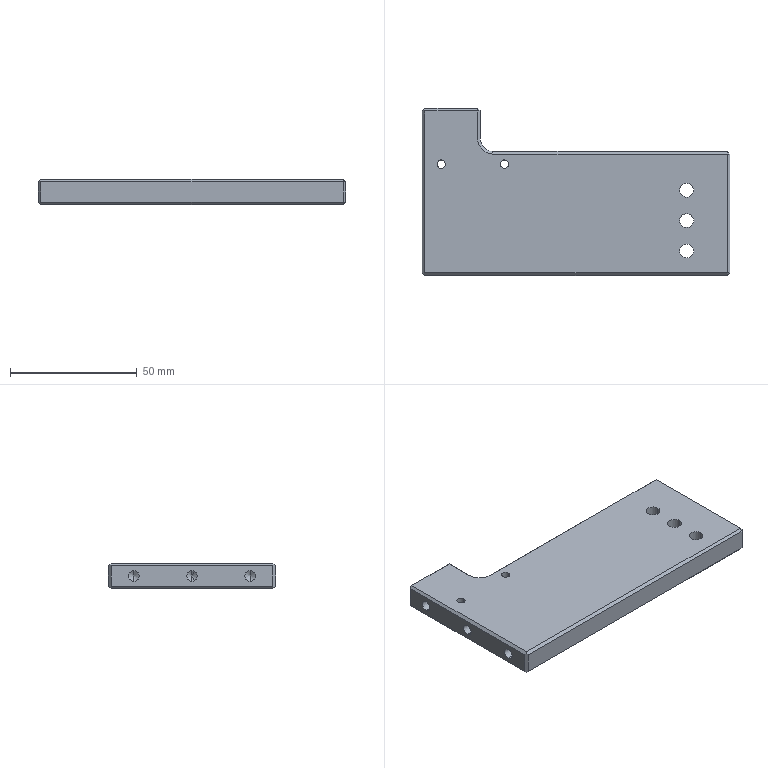Part | STEP file | 02-02 camera fixing side plate | 1 solid | 56 faces | box 121.5 x 66 x 10 mm | volume 61611 mm3 | plane 31 | cylinder 17 | cone 8 | commonest cylinder face diameters 4.2 x6 5.5 x6 3.3 x4 10 x1
STEP:
#1=CARTESIAN_POINT('',(-29.9,11.,0.));
#2=VERTEX_POINT('',#1);
#3=CARTESIAN_POINT('',(-26.6,11.,0.));
#4=VERTEX_POINT('',#3);
#5=CARTESIAN_POINT('',(-28.25,11.,0.));
#6=DIRECTION('',(0.,0.,1.));
#7=DIRECTION('',(1.,0.,0.));
#8=AXIS2_PLACEMENT_3D('',#5,#6,#7);
#9=CIRCLE('',#8,1.65);
#10=EDGE_CURVE('',#2,#4,#9,.T.);
#11=ORIENTED_EDGE('',*,*,#10,.F.);
#12=CARTESIAN_POINT('',(-29.9,11.,10.));
#13=VERTEX_POINT('',#12);
#14=CARTESIAN_POINT('',(-29.9,11.,10.));
#15=DIRECTION('',(0.,0.,1.));
#16=VECTOR('',#15,1000.);
#17=LINE('',#14,#16);
#18=EDGE_CURVE('',#2,#13,#17,.T.);
#19=ORIENTED_EDGE('',*,*,#18,.T.);
#20=CARTESIAN_POINT('',(-26.6,11.,10.));
#21=VERTEX_POINT('',#20);
#22=CARTESIAN_POINT('',(-28.25,11.,10.));
#23=DIRECTION('',(0.,0.,1.));
#24=DIRECTION('',(1.,0.,0.));
#25=AXIS2_PLACEMENT_3D('',#22,#23,#24);
#26=CIRCLE('',#25,1.65);
#27=EDGE_CURVE('',#13,#21,#26,.T.);
#28=ORIENTED_EDGE('',*,*,#27,.T.);
#29=CARTESIAN_POINT('',(-26.6,11.,10.));
#30=DIRECTION('',(0.,0.,1.));
#31=VECTOR('',#30,1000.);
#32=LINE('',#29,#31);
#33=EDGE_CURVE('',#4,#21,#32,.T.);
#34=ORIENTED_EDGE('',*,*,#33,.F.);
#35=EDGE_LOOP('',(#11,#19,#28,#34));
#36=FACE_OUTER_BOUND('',#35,.T.);
#37=CARTESIAN_POINT('',(-28.25,11.,10.));
#38=DIRECTION('',(0.,0.,1.));
#39=DIRECTION('',(1.,0.,0.));
#40=AXIS2_PLACEMENT_3D('',#37,#38,#39);
#41=CYLINDRICAL_SURFACE('',#40,1.65);
#42=ADVANCED_FACE('',(#36),#41,.F.);
#43=CARTESIAN_POINT('',(-54.9,11.,0.));
#44=VERTEX_POINT('',#43);
#45=CARTESIAN_POINT('',(-51.6,11.,0.));
#46=VERTEX_POINT('',#45);
#47=CARTESIAN_POINT('',(-53.25,11.,0.));
#48=DIRECTION('',(0.,0.,1.));
#49=DIRECTION('',(1.,0.,0.));
#50=AXIS2_PLACEMENT_3D('',#47,#48,#49);
#51=CIRCLE('',#50,1.65);
#52=EDGE_CURVE('',#44,#46,#51,.T.);
#53=ORIENTED_EDGE('',*,*,#52,.F.);
#54=CARTESIAN_POINT('',(-54.9,11.,10.));
#55=VERTEX_POINT('',#54);
#56=CARTESIAN_POINT('',(-54.9,11.,10.));
#57=DIRECTION('',(0.,0.,1.));
#58=VECTOR('',#57,1000.);
#59=LINE('',#56,#58);
#60=EDGE_CURVE('',#44,#55,#59,.T.);
#61=ORIENTED_EDGE('',*,*,#60,.T.);
#62=CARTESIAN_POINT('',(-51.6,11.,10.));
#63=VERTEX_POINT('',#62);
#64=CARTESIAN_POINT('',(-53.25,11.,10.));
#65=DIRECTION('',(0.,0.,1.));
#66=DIRECTION('',(1.,0.,0.));
#67=AXIS2_PLACEMENT_3D('',#64,#65,#66);
#68=CIRCLE('',#67,1.65);
#69=EDGE_CURVE('',#55,#63,#68,.T.);
#70=ORIENTED_EDGE('',*,*,#69,.T.);
#71=CARTESIAN_POINT('',(-51.6,11.,10.));
#72=DIRECTION('',(0.,0.,1.));
#73=VECTOR('',#72,1000.);
#74=LINE('',#71,#73);
#75=EDGE_CURVE('',#46,#63,#74,.T.);
#76=ORIENTED_EDGE('',*,*,#75,.F.);
#77=EDGE_LOOP('',(#53,#61,#70,#76));
#78=FACE_OUTER_BOUND('',#77,.T.);
#79=CARTESIAN_POINT('',(-53.25,11.,10.));
#80=DIRECTION('',(0.,0.,1.));
#81=DIRECTION('',(1.,0.,0.));
#82=AXIS2_PLACEMENT_3D('',#79,#80,#81);
#83=CYLINDRICAL_SURFACE('',#82,1.65);
#84=ADVANCED_FACE('',(#78),#83,.F.);
#85=CARTESIAN_POINT('',(-46.75,23.,2.9));
#86=VERTEX_POINT('',#85);
#87=CARTESIAN_POINT('',(-46.75,23.,7.1));
#88=VERTEX_POINT('',#87);
#89=CARTESIAN_POINT('',(-46.75,23.,5.));
#90=DIRECTION('',(-1.,0.,0.));
#91=DIRECTION('',(0.,0.,1.));
#92=AXIS2_PLACEMENT_3D('',#89,#90,#91);
#93=CIRCLE('',#92,2.1);
#94=EDGE_CURVE('',#86,#88,#93,.T.);
#95=ORIENTED_EDGE('',*,*,#94,.F.);
#96=CARTESIAN_POINT('',(-60.75,23.,2.9));
#97=VERTEX_POINT('',#96);
#98=CARTESIAN_POINT('',(-60.75,23.,2.9));
#99=DIRECTION('',(-1.,0.,0.));
#100=VECTOR('',#99,1000.);
#101=LINE('',#98,#100);
#102=EDGE_CURVE('',#86,#97,#101,.T.);
#103=ORIENTED_EDGE('',*,*,#102,.T.);
#104=CARTESIAN_POINT('',(-60.75,23.,7.1));
#105=VERTEX_POINT('',#104);
#106=CARTESIAN_POINT('',(-60.75,23.,5.));
#107=DIRECTION('',(-1.,0.,0.));
#108=DIRECTION('',(0.,0.,1.));
#109=AXIS2_PLACEMENT_3D('',#106,#107,#108);
#110=CIRCLE('',#109,2.1);
#111=EDGE_CURVE('',#97,#105,#110,.T.);
#112=ORIENTED_EDGE('',*,*,#111,.T.);
#113=CARTESIAN_POINT('',(-60.75,23.,7.1));
#114=DIRECTION('',(-1.,0.,0.));
#115=VECTOR('',#114,1000.);
#116=LINE('',#113,#115);
#117=EDGE_CURVE('',#88,#105,#116,.T.);
#118=ORIENTED_EDGE('',*,*,#117,.F.);
#119=EDGE_LOOP('',(#95,#103,#112,#118));
#120=FACE_OUTER_BOUND('',#119,.T.);
#121=CARTESIAN_POINT('',(-60.75,23.,5.));
#122=DIRECTION('',(-1.,0.,0.));
#123=DIRECTION('',(0.,0.,1.));
#124=AXIS2_PLACEMENT_3D('',#121,#122,#123);
#125=CYLINDRICAL_SURFACE('',#124,2.1);
#126=ADVANCED_FACE('',(#120),#125,.F.);
#127=CARTESIAN_POINT('',(-45.488,23.,5.));
#128=VERTEX_POINT('',#127);
#129=CARTESIAN_POINT('',(-46.75,23.,7.1));
#130=DIRECTION('',(-0.515,0.,0.8572));
#131=VECTOR('',#130,1000.);
#132=LINE('',#129,#131);
#133=EDGE_CURVE('',#128,#88,#132,.T.);
#134=ORIENTED_EDGE('',*,*,#133,.F.);
#135=CARTESIAN_POINT('',(-46.75,23.,2.9));
#136=DIRECTION('',(-0.515,0.,-0.8572));
#137=VECTOR('',#136,1000.);
#138=LINE('',#135,#137);
#139=EDGE_CURVE('',#128,#86,#138,.T.);
#140=ORIENTED_EDGE('',*,*,#139,.T.);
#141=ORIENTED_EDGE('',*,*,#94,.T.);
#142=EDGE_LOOP('',(#134,#140,#141));
#143=FACE_OUTER_BOUND('',#142,.T.);
#144=CARTESIAN_POINT('',(-46.75,23.,5.));
#145=DIRECTION('',(-1.,0.,0.));
#146=DIRECTION('',(0.,0.,1.));
#147=AXIS2_PLACEMENT_3D('',#144,#145,#146);
#148=CONICAL_SURFACE('',#147,2.1,1.03);
#149=ADVANCED_FACE('',(#143),#148,.F.);
#150=CARTESIAN_POINT('',(-46.75,0.,2.9));
#151=VERTEX_POINT('',#150);
#152=CARTESIAN_POINT('',(-46.75,0.,7.1));
#153=VERTEX_POINT('',#152);
#154=CARTESIAN_POINT('',(-46.75,0.,5.));
#155=DIRECTION('',(-1.,0.,0.));
#156=DIRECTION('',(0.,0.,1.));
#157=AXIS2_PLACEMENT_3D('',#154,#155,#156);
#158=CIRCLE('',#157,2.1);
#159=EDGE_CURVE('',#151,#153,#158,.T.);
#160=ORIENTED_EDGE('',*,*,#159,.F.);
#161=CARTESIAN_POINT('',(-60.75,0.,2.9));
#162=VERTEX_POINT('',#161);
#163=CARTESIAN_POINT('',(-60.75,0.,2.9));
#164=DIRECTION('',(-1.,0.,0.));
#165=VECTOR('',#164,1000.);
#166=LINE('',#163,#165);
#167=EDGE_CURVE('',#151,#162,#166,.T.);
#168=ORIENTED_EDGE('',*,*,#167,.T.);
#169=CARTESIAN_POINT('',(-60.75,0.,7.1));
#170=VERTEX_POINT('',#169);
#171=CARTESIAN_POINT('',(-60.75,0.,5.));
#172=DIRECTION('',(-1.,0.,0.));
#173=DIRECTION('',(0.,0.,1.));
#174=AXIS2_PLACEMENT_3D('',#171,#172,#173);
#175=CIRCLE('',#174,2.1);
#176=EDGE_CURVE('',#162,#170,#175,.T.);
#177=ORIENTED_EDGE('',*,*,#176,.T.);
#178=CARTESIAN_POINT('',(-60.75,0.,7.1));
#179=DIRECTION('',(-1.,0.,0.));
#180=VECTOR('',#179,1000.);
#181=LINE('',#178,#180);
#182=EDGE_CURVE('',#153,#170,#181,.T.);
#183=ORIENTED_EDGE('',*,*,#182,.F.);
#184=EDGE_LOOP('',(#160,#168,#177,#183));
#185=FACE_OUTER_BOUND('',#184,.T.);
#186=CARTESIAN_POINT('',(-60.75,0.,5.));
#187=DIRECTION('',(-1.,0.,0.));
#188=DIRECTION('',(0.,0.,1.));
#189=AXIS2_PLACEMENT_3D('',#186,#187,#188);
#190=CYLINDRICAL_SURFACE('',#189,2.1);
#191=ADVANCED_FACE('',(#185),#190,.F.);
#192=CARTESIAN_POINT('',(-45.488,0.,5.));
#193=VERTEX_POINT('',#192);
#194=CARTESIAN_POINT('',(-46.75,0.,7.1));
#195=DIRECTION('',(-0.515,0.,0.8572));
#196=VECTOR('',#195,1000.);
#197=LINE('',#194,#196);
#198=EDGE_CURVE('',#193,#153,#197,.T.);
#199=ORIENTED_EDGE('',*,*,#198,.F.);
#200=CARTESIAN_POINT('',(-46.75,0.,2.9));
#201=DIRECTION('',(-0.515,0.,-0.8572));
#202=VECTOR('',#201,1000.);
#203=LINE('',#200,#202);
#204=EDGE_CURVE('',#193,#151,#203,.T.);
#205=ORIENTED_EDGE('',*,*,#204,.T.);
#206=ORIENTED_EDGE('',*,*,#159,.T.);
#207=EDGE_LOOP('',(#199,#205,#206));
#208=FACE_OUTER_BOUND('',#207,.T.);
#209=CARTESIAN_POINT('',(-46.75,0.,5.));
#210=DIRECTION('',(-1.,0.,0.));
#211=DIRECTION('',(0.,0.,1.));
#212=AXIS2_PLACEMENT_3D('',#209,#210,#211);
#213=CONICAL_SURFACE('',#212,2.1,1.03);
#214=ADVANCED_FACE('',(#208),#213,.F.);
#215=CARTESIAN_POINT('',(-46.75,-23.,2.9));
#216=VERTEX_POINT('',#215);
#217=CARTESIAN_POINT('',(-46.75,-23.,7.1));
#218=VERTEX_POINT('',#217);
#219=CARTESIAN_POINT('',(-46.75,-23.,5.));
#220=DIRECTION('',(-1.,0.,0.));
#221=DIRECTION('',(0.,0.,1.));
#222=AXIS2_PLACEMENT_3D('',#219,#220,#221);
#223=CIRCLE('',#222,2.1);
#224=EDGE_CURVE('',#216,#218,#223,.T.);
#225=ORIENTED_EDGE('',*,*,#224,.F.);
#226=CARTESIAN_POINT('',(-60.75,-23.,2.9));
#227=VERTEX_POINT('',#226);
#228=CARTESIAN_POINT('',(-60.75,-23.,2.9));
#229=DIRECTION('',(-1.,0.,0.));
#230=VECTOR('',#229,1000.);
#231=LINE('',#228,#230);
#232=EDGE_CURVE('',#216,#227,#231,.T.);
#233=ORIENTED_EDGE('',*,*,#232,.T.);
#234=CARTESIAN_POINT('',(-60.75,-23.,7.1));
#235=VERTEX_POINT('',#234);
#236=CARTESIAN_POINT('',(-60.75,-23.,5.));
#237=DIRECTION('',(-1.,0.,0.));
#238=DIRECTION('',(0.,0.,1.));
#239=AXIS2_PLACEMENT_3D('',#236,#237,#238);
#240=CIRCLE('',#239,2.1);
#241=EDGE_CURVE('',#227,#235,#240,.T.);
#242=ORIENTED_EDGE('',*,*,#241,.T.);
#243=CARTESIAN_POINT('',(-60.75,-23.,7.1));
#244=DIRECTION('',(-1.,0.,0.));
#245=VECTOR('',#244,1000.);
#246=LINE('',#243,#245);
#247=EDGE_CURVE('',#218,#235,#246,.T.);
#248=ORIENTED_EDGE('',*,*,#247,.F.);
#249=EDGE_LOOP('',(#225,#233,#242,#248));
#250=FACE_OUTER_BOUND('',#249,.T.);
#251=CARTESIAN_POINT('',(-60.75,-23.,5.));
#252=DIRECTION('',(-1.,0.,0.));
#253=DIRECTION('',(0.,0.,1.));
#254=AXIS2_PLACEMENT_3D('',#251,#252,#253);
#255=CYLINDRICAL_SURFACE('',#254,2.1);
#256=ADVANCED_FACE('',(#250),#255,.F.);
#257=CARTESIAN_POINT('',(-45.488,-23.,5.));
#258=VERTEX_POINT('',#257);
#259=CARTESIAN_POINT('',(-46.75,-23.,7.1));
#260=DIRECTION('',(-0.515,0.,0.8572));
#261=VECTOR('',#260,1000.);
#262=LINE('',#259,#261);
#263=EDGE_CURVE('',#258,#218,#262,.T.);
#264=ORIENTED_EDGE('',*,*,#263,.F.);
#265=CARTESIAN_POINT('',(-46.75,-23.,2.9));
#266=DIRECTION('',(-0.515,0.,-0.8572));
#267=VECTOR('',#266,1000.);
#268=LINE('',#265,#267);
#269=EDGE_CURVE('',#258,#216,#268,.T.);
#270=ORIENTED_EDGE('',*,*,#269,.T.);
#271=ORIENTED_EDGE('',*,*,#224,.T.);
#272=EDGE_LOOP('',(#264,#270,#271));
#273=FACE_OUTER_BOUND('',#272,.T.);
#274=CARTESIAN_POINT('',(-46.75,-23.,5.));
#275=DIRECTION('',(-1.,0.,0.));
#276=DIRECTION('',(0.,0.,1.));
#277=AXIS2_PLACEMENT_3D('',#274,#275,#276);
#278=CONICAL_SURFACE('',#277,2.1,1.03);
#279=ADVANCED_FACE('',(#273),#278,.F.);
#280=CARTESIAN_POINT('',(46.5,-23.3,10.));
#281=VERTEX_POINT('',#280);
#282=CARTESIAN_POINT('',(41.,-23.3,10.));
#283=VERTEX_POINT('',#282);
#284=CARTESIAN_POINT('',(43.75,-23.3,10.));
#285=DIRECTION('',(0.,0.,-1.));
#286=DIRECTION('',(-1.,0.,0.));
#287=AXIS2_PLACEMENT_3D('',#284,#285,#286);
#288=CIRCLE('',#287,2.75);
#289=EDGE_CURVE('',#281,#283,#288,.T.);
#290=ORIENTED_EDGE('',*,*,#289,.F.);
#291=CARTESIAN_POINT('',(46.5,-23.3,0.));
#292=VERTEX_POINT('',#291);
#293=CARTESIAN_POINT('',(46.5,-23.3,10.));
#294=DIRECTION('',(0.,0.,-1.));
#295=VECTOR('',#294,1000.);
#296=LINE('',#293,#295);
#297=EDGE_CURVE('',#281,#292,#296,.T.);
#298=ORIENTED_EDGE('',*,*,#297,.T.);
#299=CARTESIAN_POINT('',(41.,-23.3,0.));
#300=VERTEX_POINT('',#299);
#301=CARTESIAN_POINT('',(43.75,-23.3,0.));
#302=DIRECTION('',(0.,0.,-1.));
#303=DIRECTION('',(-1.,0.,0.));
#304=AXIS2_PLACEMENT_3D('',#301,#302,#303);
#305=CIRCLE('',#304,2.75);
#306=EDGE_CURVE('',#292,#300,#305,.T.);
#307=ORIENTED_EDGE('',*,*,#306,.T.);
#308=CARTESIAN_POINT('',(41.,-23.3,10.));
#309=DIRECTION('',(0.,0.,-1.));
#310=VECTOR('',#309,1000.);
#311=LINE('',#308,#310);
#312=EDGE_CURVE('',#283,#300,#311,.T.);
#313=ORIENTED_EDGE('',*,*,#312,.F.);
#314=EDGE_LOOP('',(#290,#298,#307,#313));
#315=FACE_OUTER_BOUND('',#314,.T.);
#316=CARTESIAN_POINT('',(43.75,-23.3,10.));
#317=DIRECTION('',(0.,0.,-1.));
#318=DIRECTION('',(-1.,0.,0.));
#319=AXIS2_PLACEMENT_3D('',#316,#317,#318);
#320=CYLINDRICAL_SURFACE('',#319,2.75);
#321=ADVANCED_FACE('',(#315),#320,.F.);
#322=CARTESIAN_POINT('',(46.5,-11.3,10.));
#323=VERTEX_POINT('',#322);
#324=CARTESIAN_POINT('',(41.,-11.3,10.));
#325=VERTEX_POINT('',#324);
#326=CARTESIAN_POINT('',(43.75,-11.3,10.));
#327=DIRECTION('',(0.,0.,-1.));
#328=DIRECTION('',(-1.,0.,0.));
#329=AXIS2_PLACEMENT_3D('',#326,#327,#328);
#330=CIRCLE('',#329,2.75);
#331=EDGE_CURVE('',#323,#325,#330,.T.);
#332=ORIENTED_EDGE('',*,*,#331,.F.);
#333=CARTESIAN_POINT('',(46.5,-11.3,0.));
#334=VERTEX_POINT('',#333);
#335=CARTESIAN_POINT('',(46.5,-11.3,10.));
#336=DIRECTION('',(0.,0.,-1.));
#337=VECTOR('',#336,1000.);
#338=LINE('',#335,#337);
#339=EDGE_CURVE('',#323,#334,#338,.T.);
#340=ORIENTED_EDGE('',*,*,#339,.T.);
#341=CARTESIAN_POINT('',(41.,-11.3,0.));
#342=VERTEX_POINT('',#341);
#343=CARTESIAN_POINT('',(43.75,-11.3,0.));
#344=DIRECTION('',(0.,0.,-1.));
#345=DIRECTION('',(-1.,0.,0.));
#346=AXIS2_PLACEMENT_3D('',#343,#344,#345);
#347=CIRCLE('',#346,2.75);
#348=EDGE_CURVE('',#334,#342,#347,.T.);
#349=ORIENTED_EDGE('',*,*,#348,.T.);
#350=CARTESIAN_POINT('',(41.,-11.3,10.));
#351=DIRECTION('',(0.,0.,-1.));
#352=VECTOR('',#351,1000.);
#353=LINE('',#350,#352);
#354=EDGE_CURVE('',#325,#342,#353,.T.);
#355=ORIENTED_EDGE('',*,*,#354,.F.);
#356=EDGE_LOOP('',(#332,#340,#349,#355));
#357=FACE_OUTER_BOUND('',#356,.T.);
#358=CARTESIAN_POINT('',(43.75,-11.3,10.));
#359=DIRECTION('',(0.,0.,-1.));
#360=DIRECTION('',(-1.,0.,0.));
#361=AXIS2_PLACEMENT_3D('',#358,#359,#360);
#362=CYLINDRICAL_SURFACE('',#361,2.75);
#363=ADVANCED_FACE('',(#357),#362,.F.);
#364=CARTESIAN_POINT('',(46.5,0.7,10.));
#365=VERTEX_POINT('',#364);
#366=CARTESIAN_POINT('',(41.,0.7,10.));
#367=VERTEX_POINT('',#366);
#368=CARTESIAN_POINT('',(43.75,0.7,10.));
#369=DIRECTION('',(0.,0.,-1.));
#370=DIRECTION('',(-1.,0.,0.));
#371=AXIS2_PLACEMENT_3D('',#368,#369,#370);
#372=CIRCLE('',#371,2.75);
#373=EDGE_CURVE('',#365,#367,#372,.T.);
#374=ORIENTED_EDGE('',*,*,#373,.F.);
#375=CARTESIAN_POINT('',(46.5,0.7,0.));
#376=VERTEX_POINT('',#375);
#377=CARTESIAN_POINT('',(46.5,0.7,10.));
#378=DIRECTION('',(0.,0.,-1.));
#379=VECTOR('',#378,1000.);
#380=LINE('',#377,#379);
#381=EDGE_CURVE('',#365,#376,#380,.T.);
#382=ORIENTED_EDGE('',*,*,#381,.T.);
#383=CARTESIAN_POINT('',(41.,0.7,0.));
#384=VERTEX_POINT('',#383);
#385=CARTESIAN_POINT('',(43.75,0.7,0.));
#386=DIRECTION('',(0.,0.,-1.));
#387=DIRECTION('',(-1.,0.,0.));
#388=AXIS2_PLACEMENT_3D('',#385,#386,#387);
#389=CIRCLE('',#388,2.75);
#390=EDGE_CURVE('',#376,#384,#389,.T.);
#391=ORIENTED_EDGE('',*,*,#390,.T.);
#392=CARTESIAN_POINT('',(41.,0.7,10.));
#393=DIRECTION('',(0.,0.,-1.));
#394=VECTOR('',#393,1000.);
#395=LINE('',#392,#394);
#396=EDGE_CURVE('',#367,#384,#395,.T.);
#397=ORIENTED_EDGE('',*,*,#396,.F.);
#398=EDGE_LOOP('',(#374,#382,#391,#397));
#399=FACE_OUTER_BOUND('',#398,.T.);
#400=CARTESIAN_POINT('',(43.75,0.7,10.));
#401=DIRECTION('',(0.,0.,-1.));
#402=DIRECTION('',(-1.,0.,0.));
#403=AXIS2_PLACEMENT_3D('',#400,#401,#402);
#404=CYLINDRICAL_SURFACE('',#403,2.75);
#405=ADVANCED_FACE('',(#399),#404,.F.);
#406=CARTESIAN_POINT('',(60.75,15.,1.));
#407=VERTEX_POINT('',#406);
#408=CARTESIAN_POINT('',(60.75,15.,9.));
#409=VERTEX_POINT('',#408);
#410=CARTESIAN_POINT('',(60.75,15.,10.));
#411=DIRECTION('',(0.,0.,1.));
#412=VECTOR('',#411,1000.);
#413=LINE('',#410,#412);
#414=EDGE_CURVE('',#407,#409,#413,.T.);
#415=ORIENTED_EDGE('',*,*,#414,.T.);
#416=CARTESIAN_POINT('',(60.75,-32.,9.));
#417=VERTEX_POINT('',#416);
#418=CARTESIAN_POINT('',(60.75,-33.,9.));
#419=DIRECTION('',(0.,-1.,0.));
#420=VECTOR('',#419,1000.);
#421=LINE('',#418,#420);
#422=EDGE_CURVE('',#409,#417,#421,.T.);
#423=ORIENTED_EDGE('',*,*,#422,.T.);
#424=CARTESIAN_POINT('',(60.75,-32.,1.));
#425=VERTEX_POINT('',#424);
#426=CARTESIAN_POINT('',(60.75,-32.,10.));
#427=DIRECTION('',(0.,0.,-1.));
#428=VECTOR('',#427,1000.);
#429=LINE('',#426,#428);
#430=EDGE_CURVE('',#417,#425,#429,.T.);
#431=ORIENTED_EDGE('',*,*,#430,.T.);
#432=CARTESIAN_POINT('',(60.75,33.,1.));
#433=DIRECTION('',(0.,1.,0.));
#434=VECTOR('',#433,1000.);
#435=LINE('',#432,#434);
#436=EDGE_CURVE('',#425,#407,#435,.T.);
#437=ORIENTED_EDGE('',*,*,#436,.T.);
#438=EDGE_LOOP('',(#415,#423,#431,#437));
#439=FACE_OUTER_BOUND('',#438,.T.);
#440=CARTESIAN_POINT('',(60.75,33.,10.));
#441=DIRECTION('',(-1.,0.,0.));
#442=DIRECTION('',(0.,-1.,0.));
#443=AXIS2_PLACEMENT_3D('',#440,#441,#442);
#444=PLANE('',#443);
#445=ADVANCED_FACE('',(#439),#444,.F.);
#446=CARTESIAN_POINT('',(-38.827,33.,1.));
#447=VERTEX_POINT('',#446);
#448=CARTESIAN_POINT('',(-59.75,33.,1.));
#449=VERTEX_POINT('',#448);
#450=CARTESIAN_POINT('',(-60.75,33.,1.));
#451=DIRECTION('',(-1.,0.,0.));
#452=VECTOR('',#451,1000.);
#453=LINE('',#450,#452);
#454=EDGE_CURVE('',#447,#449,#453,.T.);
#455=ORIENTED_EDGE('',*,*,#454,.T.);
#456=CARTESIAN_POINT('',(-59.75,33.,9.));
#457=VERTEX_POINT('',#456);
#458=CARTESIAN_POINT('',(-59.75,33.,10.));
#459=DIRECTION('',(0.,0.,1.));
#460=VECTOR('',#459,1000.);
#461=LINE('',#458,#460);
#462=EDGE_CURVE('',#449,#457,#461,.T.);
#463=ORIENTED_EDGE('',*,*,#462,.T.);
#464=CARTESIAN_POINT('',(-38.827,33.,9.));
#465=VERTEX_POINT('',#464);
#466=CARTESIAN_POINT('',(-37.827,33.,9.));
#467=DIRECTION('',(1.,0.,0.));
#468=VECTOR('',#467,1000.);
#469=LINE('',#466,#468);
#470=EDGE_CURVE('',#457,#465,#469,.T.);
#471=ORIENTED_EDGE('',*,*,#470,.T.);
#472=CARTESIAN_POINT('',(-38.827,33.,10.));
#473=DIRECTION('',(0.,0.,-1.));
#474=VECTOR('',#473,1000.);
#475=LINE('',#472,#474);
#476=EDGE_CURVE('',#465,#447,#475,.T.);
#477=ORIENTED_EDGE('',*,*,#476,.T.);
#478=EDGE_LOOP('',(#455,#463,#471,#477));
#479=FACE_OUTER_BOUND('',#478,.T.);
#480=CARTESIAN_POINT('',(-60.75,33.,10.));
#481=DIRECTION('',(0.,-1.,0.));
#482=DIRECTION('',(0.,0.,-1.));
#483=AXIS2_PLACEMENT_3D('',#480,#481,#482);
#484=PLANE('',#483);
#485=ADVANCED_FACE('',(#479),#484,.F.);
#486=CARTESIAN_POINT('',(-60.75,23.,5.));
#487=DIRECTION('',(-1.,0.,0.));
#488=DIRECTION('',(0.,0.,1.));
#489=AXIS2_PLACEMENT_3D('',#486,#487,#488);
#490=CIRCLE('',#489,2.1);
#491=EDGE_CURVE('',#105,#97,#490,.T.);
#492=ORIENTED_EDGE('',*,*,#491,.F.);
#493=ORIENTED_EDGE('',*,*,#111,.F.);
#494=EDGE_LOOP('',(#492,#493));
#495=FACE_BOUND('',#494,.T.);
#496=CARTESIAN_POINT('',(-60.75,0.,5.));
#497=DIRECTION('',(-1.,0.,0.));
#498=DIRECTION('',(0.,0.,1.));
#499=AXIS2_PLACEMENT_3D('',#496,#497,#498);
#500=CIRCLE('',#499,2.1);
#501=EDGE_CURVE('',#170,#162,#500,.T.);
#502=ORIENTED_EDGE('',*,*,#501,.F.);
#503=ORIENTED_EDGE('',*,*,#176,.F.);
#504=EDGE_LOOP('',(#502,#503));
#505=FACE_BOUND('',#504,.T.);
#506=CARTESIAN_POINT('',(-60.75,-23.,5.));
#507=DIRECTION('',(-1.,0.,0.));
#508=DIRECTION('',(0.,0.,1.));
#509=AXIS2_PLACEMENT_3D('',#506,#507,#508);
#510=CIRCLE('',#509,2.1);
#511=EDGE_CURVE('',#235,#227,#510,.T.);
#512=ORIENTED_EDGE('',*,*,#511,.F.);
#513=ORIENTED_EDGE('',*,*,#241,.F.);
#514=EDGE_LOOP('',(#512,#513));
#515=FACE_BOUND('',#514,.T.);
#516=CARTESIAN_POINT('',(-60.75,-32.,1.));
#517=VERTEX_POINT('',#516);
#518=CARTESIAN_POINT('',(-60.75,-32.,9.));
#519=VERTEX_POINT('',#518);
#520=CARTESIAN_POINT('',(-60.75,-32.,10.));
#521=DIRECTION('',(0.,0.,1.));
#522=VECTOR('',#521,1000.);
#523=LINE('',#520,#522);
#524=EDGE_CURVE('',#517,#519,#523,.T.);
#525=ORIENTED_EDGE('',*,*,#524,.T.);
#526=CARTESIAN_POINT('',(-60.75,32.,9.));
#527=VERTEX_POINT('',#526);
#528=CARTESIAN_POINT('',(-60.75,32.,9.));
#529=DIRECTION('',(0.,1.,0.));
#530=VECTOR('',#529,1000.);
#531=LINE('',#528,#530);
#532=EDGE_CURVE('',#519,#527,#531,.T.);
#533=ORIENTED_EDGE('',*,*,#532,.T.);
#534=CARTESIAN_POINT('',(-60.75,32.,1.));
#535=VERTEX_POINT('',#534);
#536=CARTESIAN_POINT('',(-60.75,32.,10.));
#537=DIRECTION('',(0.,0.,-1.));
#538=VECTOR('',#537,1000.);
#539=LINE('',#536,#538);
#540=EDGE_CURVE('',#527,#535,#539,.T.);
#541=ORIENTED_EDGE('',*,*,#540,.T.);
#542=CARTESIAN_POINT('',(-60.75,33.,1.));
#543=DIRECTION('',(0.,-1.,0.));
#544=VECTOR('',#543,1000.);
#545=LINE('',#542,#544);
#546=EDGE_CURVE('',#535,#517,#545,.T.);
#547=ORIENTED_EDGE('',*,*,#546,.T.);
#548=EDGE_LOOP('',(#525,#533,#541,#547));
#549=FACE_OUTER_BOUND('',#548,.T.);
#550=CARTESIAN_POINT('',(-60.75,33.,10.));
#551=DIRECTION('',(1.,0.,0.));
#552=DIRECTION('',(0.,1.,0.));
#553=AXIS2_PLACEMENT_3D('',#550,#551,#552);
#554=PLANE('',#553);
#555=ADVANCED_FACE('',(#495,#505,#515,#549),#554,.F.);
#556=CARTESIAN_POINT('',(59.75,-33.,9.));
#557=VERTEX_POINT('',#556);
#558=CARTESIAN_POINT('',(-59.75,-33.,9.));
#559=VERTEX_POINT('',#558);
#560=CARTESIAN_POINT('',(-60.75,-33.,9.));
#561=DIRECTION('',(-1.,0.,0.));
#562=VECTOR('',#561,1000.);
#563=LINE('',#560,#562);
#564=EDGE_CURVE('',#557,#559,#563,.T.);
#565=ORIENTED_EDGE('',*,*,#564,.T.);
#566=CARTESIAN_POINT('',(-59.75,-33.,1.));
#567=VERTEX_POINT('',#566);
#568=CARTESIAN_POINT('',(-59.75,-33.,10.));
#569=DIRECTION('',(0.,0.,-1.));
#570=VECTOR('',#569,1000.);
#571=LINE('',#568,#570);
#572=EDGE_CURVE('',#559,#567,#571,.T.);
#573=ORIENTED_EDGE('',*,*,#572,.T.);
#574=CARTESIAN_POINT('',(59.75,-33.,1.));
#575=VERTEX_POINT('',#574);
#576=CARTESIAN_POINT('',(-60.75,-33.,1.));
#577=DIRECTION('',(1.,0.,0.));
#578=VECTOR('',#577,1000.);
#579=LINE('',#576,#578);
#580=EDGE_CURVE('',#567,#575,#579,.T.);
#581=ORIENTED_EDGE('',*,*,#580,.T.);
#582=CARTESIAN_POINT('',(59.75,-33.,10.));
#583=DIRECTION('',(0.,0.,1.));
#584=VECTOR('',#583,1000.);
#585=LINE('',#582,#584);
#586=EDGE_CURVE('',#575,#557,#585,.T.);
#587=ORIENTED_EDGE('',*,*,#586,.T.);
#588=EDGE_LOOP('',(#565,#573,#581,#587));
#589=FACE_OUTER_BOUND('',#588,.T.);
#590=CARTESIAN_POINT('',(-60.75,-33.,10.));
#591=DIRECTION('',(0.,1.,0.));
#592=DIRECTION('',(0.,0.,1.));
#593=AXIS2_PLACEMENT_3D('',#590,#591,#592);
#594=PLANE('',#593);
#595=ADVANCED_FACE('',(#589),#594,.F.);
#596=CARTESIAN_POINT('',(-28.25,11.,10.));
#597=DIRECTION('',(0.,0.,1.));
#598=DIRECTION('',(1.,0.,0.));
#599=AXIS2_PLACEMENT_3D('',#596,#597,#598);
#600=CIRCLE('',#599,1.65);
#601=EDGE_CURVE('',#21,#13,#600,.T.);
#602=ORIENTED_EDGE('',*,*,#601,.F.);
#603=ORIENTED_EDGE('',*,*,#27,.F.);
#604=EDGE_LOOP('',(#602,#603));
#605=FACE_BOUND('',#604,.T.);
#606=CARTESIAN_POINT('',(-53.25,11.,10.));
#607=DIRECTION('',(0.,0.,1.));
#608=DIRECTION('',(1.,0.,0.));
#609=AXIS2_PLACEMENT_3D('',#606,#607,#608);
#610=CIRCLE('',#609,1.65);
#611=EDGE_CURVE('',#63,#55,#610,.T.);
#612=ORIENTED_EDGE('',*,*,#611,.F.);
#613=ORIENTED_EDGE('',*,*,#69,.F.);
#614=EDGE_LOOP('',(#612,#613));
#615=FACE_BOUND('',#614,.T.);
#616=CARTESIAN_POINT('',(-38.827,32.,10.));
#617=VERTEX_POINT('',#616);
#618=CARTESIAN_POINT('',(-59.75,32.,10.));
#619=VERTEX_POINT('',#618);
#620=CARTESIAN_POINT('',(-60.75,32.,10.));
#621=DIRECTION('',(-1.,0.,0.));
#622=VECTOR('',#621,1000.);
#623=LINE('',#620,#622);
#624=EDGE_CURVE('',#617,#619,#623,.T.);
#625=ORIENTED_EDGE('',*,*,#624,.T.);
#626=CARTESIAN_POINT('',(-59.75,-32.,10.));
#627=VERTEX_POINT('',#626);
#628=CARTESIAN_POINT('',(-59.75,-32.,10.));
#629=DIRECTION('',(0.,-1.,0.));
#630=VECTOR('',#629,1000.);
#631=LINE('',#628,#630);
#632=EDGE_CURVE('',#619,#627,#631,.T.);
#633=ORIENTED_EDGE('',*,*,#632,.T.);
#634=CARTESIAN_POINT('',(59.75,-32.,10.));
#635=VERTEX_POINT('',#634);
#636=CARTESIAN_POINT('',(60.75,-32.,10.));
#637=DIRECTION('',(1.,0.,0.));
#638=VECTOR('',#637,1000.);
#639=LINE('',#636,#638);
#640=EDGE_CURVE('',#627,#635,#639,.T.);
#641=ORIENTED_EDGE('',*,*,#640,.T.);
#642=CARTESIAN_POINT('',(59.75,15.,10.));
#643=VERTEX_POINT('',#642);
#644=CARTESIAN_POINT('',(59.75,16.,10.));
#645=DIRECTION('',(0.,1.,0.));
#646=VECTOR('',#645,1000.);
#647=LINE('',#644,#646);
#648=EDGE_CURVE('',#635,#643,#647,.T.);
#649=ORIENTED_EDGE('',*,*,#648,.T.);
#650=CARTESIAN_POINT('',(-32.827,15.,10.));
#651=VERTEX_POINT('',#650);
#652=CARTESIAN_POINT('',(-32.827,15.,10.));
#653=DIRECTION('',(-1.,0.,0.));
#654=VECTOR('',#653,1000.);
#655=LINE('',#652,#654);
#656=EDGE_CURVE('',#643,#651,#655,.T.);
#657=ORIENTED_EDGE('',*,*,#656,.T.);
#658=CARTESIAN_POINT('',(-38.827,21.,10.));
#659=VERTEX_POINT('',#658);
#660=CARTESIAN_POINT('',(-32.827,21.,10.));
#661=DIRECTION('',(0.,0.,-1.));
#662=DIRECTION('',(1.,0.,0.));
#663=AXIS2_PLACEMENT_3D('',#660,#661,#662);
#664=CIRCLE('',#663,6.);
#665=EDGE_CURVE('',#651,#659,#664,.T.);
#666=ORIENTED_EDGE('',*,*,#665,.T.);
#667=CARTESIAN_POINT('',(-38.827,33.,10.));
#668=DIRECTION('',(0.,1.,0.));
#669=VECTOR('',#668,1000.);
#670=LINE('',#667,#669);
#671=EDGE_CURVE('',#659,#617,#670,.T.);
#672=ORIENTED_EDGE('',*,*,#671,.T.);
#673=EDGE_LOOP('',(#625,#633,#641,#649,#657,#666,#672));
#674=FACE_OUTER_BOUND('',#673,.T.);
#675=CARTESIAN_POINT('',(43.75,-23.3,10.));
#676=DIRECTION('',(0.,0.,-1.));
#677=DIRECTION('',(-1.,0.,0.));
#678=AXIS2_PLACEMENT_3D('',#675,#676,#677);
#679=CIRCLE('',#678,2.75);
#680=EDGE_CURVE('',#283,#281,#679,.T.);
#681=ORIENTED_EDGE('',*,*,#680,.T.);
#682=ORIENTED_EDGE('',*,*,#289,.T.);
#683=EDGE_LOOP('',(#681,#682));
#684=FACE_BOUND('',#683,.T.);
#685=CARTESIAN_POINT('',(43.75,-11.3,10.));
#686=DIRECTION('',(0.,0.,-1.));
#687=DIRECTION('',(-1.,0.,0.));
#688=AXIS2_PLACEMENT_3D('',#685,#686,#687);
#689=CIRCLE('',#688,2.75);
#690=EDGE_CURVE('',#325,#323,#689,.T.);
#691=ORIENTED_EDGE('',*,*,#690,.T.);
#692=ORIENTED_EDGE('',*,*,#331,.T.);
#693=EDGE_LOOP('',(#691,#692));
#694=FACE_BOUND('',#693,.T.);
#695=CARTESIAN_POINT('',(43.75,0.7,10.));
#696=DIRECTION('',(0.,0.,-1.));
#697=DIRECTION('',(-1.,0.,0.));
#698=AXIS2_PLACEMENT_3D('',#695,#696,#697);
#699=CIRCLE('',#698,2.75);
#700=EDGE_CURVE('',#367,#365,#699,.T.);
#701=ORIENTED_EDGE('',*,*,#700,.T.);
#702=ORIENTED_EDGE('',*,*,#373,.T.);
#703=EDGE_LOOP('',(#701,#702));
#704=FACE_BOUND('',#703,.T.);
#705=CARTESIAN_POINT('',(60.75,-33.,10.));
#706=DIRECTION('',(0.,0.,1.));
#707=DIRECTION('',(1.,0.,0.));
#708=AXIS2_PLACEMENT_3D('',#705,#706,#707);
#709=PLANE('',#708);
#710=ADVANCED_FACE('',(#605,#615,#674,#684,#694,#704),#709,.T.);
#711=CARTESIAN_POINT('',(-28.25,11.,0.));
#712=DIRECTION('',(0.,0.,1.));
#713=DIRECTION('',(1.,0.,0.));
#714=AXIS2_PLACEMENT_3D('',#711,#712,#713);
#715=CIRCLE('',#714,1.65);
#716=EDGE_CURVE('',#4,#2,#715,.T.);
#717=ORIENTED_EDGE('',*,*,#716,.T.);
#718=ORIENTED_EDGE('',*,*,#10,.T.);
#719=EDGE_LOOP('',(#717,#718));
#720=FACE_BOUND('',#719,.T.);
#721=CARTESIAN_POINT('',(-53.25,11.,0.));
#722=DIRECTION('',(0.,0.,1.));
#723=DIRECTION('',(1.,0.,0.));
#724=AXIS2_PLACEMENT_3D('',#721,#722,#723);
#725=CIRCLE('',#724,1.65);
#726=EDGE_CURVE('',#46,#44,#725,.T.);
#727=ORIENTED_EDGE('',*,*,#726,.T.);
#728=ORIENTED_EDGE('',*,*,#52,.T.);
#729=EDGE_LOOP('',(#727,#728));
#730=FACE_BOUND('',#729,.T.);
#731=CARTESIAN_POINT('',(43.75,-23.3,0.));
#732=DIRECTION('',(0.,0.,-1.));
#733=DIRECTION('',(-1.,0.,0.));
#734=AXIS2_PLACEMENT_3D('',#731,#732,#733);
#735=CIRCLE('',#734,2.75);
#736=EDGE_CURVE('',#300,#292,#735,.T.);
#737=ORIENTED_EDGE('',*,*,#736,.F.);
#738=ORIENTED_EDGE('',*,*,#306,.F.);
#739=EDGE_LOOP('',(#737,#738));
#740=FACE_BOUND('',#739,.T.);
#741=CARTESIAN_POINT('',(43.75,-11.3,0.));
#742=DIRECTION('',(0.,0.,-1.));
#743=DIRECTION('',(-1.,0.,0.));
#744=AXIS2_PLACEMENT_3D('',#741,#742,#743);
#745=CIRCLE('',#744,2.75);
#746=EDGE_CURVE('',#342,#334,#745,.T.);
#747=ORIENTED_EDGE('',*,*,#746,.F.);
#748=ORIENTED_EDGE('',*,*,#348,.F.);
#749=EDGE_LOOP('',(#747,#748));
#750=FACE_BOUND('',#749,.T.);
#751=CARTESIAN_POINT('',(43.75,0.7,0.));
#752=DIRECTION('',(0.,0.,-1.));
#753=DIRECTION('',(-1.,0.,0.));
#754=AXIS2_PLACEMENT_3D('',#751,#752,#753);
#755=CIRCLE('',#754,2.75);
#756=EDGE_CURVE('',#384,#376,#755,.T.);
#757=ORIENTED_EDGE('',*,*,#756,.F.);
#758=ORIENTED_EDGE('',*,*,#390,.F.);
#759=EDGE_LOOP('',(#757,#758));
#760=FACE_BOUND('',#759,.T.);
#761=CARTESIAN_POINT('',(59.75,-32.,0.));
#762=VERTEX_POINT('',#761);
#763=CARTESIAN_POINT('',(-59.75,-32.,0.));
#764=VERTEX_POINT('',#763);
#765=CARTESIAN_POINT('',(60.75,-32.,0.));
#766=DIRECTION('',(-1.,0.,0.));
#767=VECTOR('',#766,1000.);
#768=LINE('',#765,#767);
#769=EDGE_CURVE('',#762,#764,#768,.T.);
#770=ORIENTED_EDGE('',*,*,#769,.T.);
#771=CARTESIAN_POINT('',(-59.75,32.,0.));
#772=VERTEX_POINT('',#771);
#773=CARTESIAN_POINT('',(-59.75,-33.,0.));
#774=DIRECTION('',(0.,1.,0.));
#775=VECTOR('',#774,1000.);
#776=LINE('',#773,#775);
#777=EDGE_CURVE('',#764,#772,#776,.T.);
#778=ORIENTED_EDGE('',*,*,#777,.T.);
#779=CARTESIAN_POINT('',(-38.827,32.,0.));
#780=VERTEX_POINT('',#779);
#781=CARTESIAN_POINT('',(60.75,32.,0.));
#782=DIRECTION('',(1.,0.,0.));
#783=VECTOR('',#782,1000.);
#784=LINE('',#781,#783);
#785=EDGE_CURVE('',#772,#780,#784,.T.);
#786=ORIENTED_EDGE('',*,*,#785,.T.);
#787=CARTESIAN_POINT('',(-38.827,21.,0.));
#788=VERTEX_POINT('',#787);
#789=CARTESIAN_POINT('',(-38.827,-33.,0.));
#790=DIRECTION('',(0.,-1.,0.));
#791=VECTOR('',#790,1000.);
#792=LINE('',#789,#791);
#793=EDGE_CURVE('',#780,#788,#792,.T.);
#794=ORIENTED_EDGE('',*,*,#793,.T.);
#795=CARTESIAN_POINT('',(-32.827,15.,0.));
#796=VERTEX_POINT('',#795);
#797=CARTESIAN_POINT('',(-32.827,21.,0.));
#798=DIRECTION('',(0.,0.,1.));
#799=DIRECTION('',(1.,0.,0.));
#800=AXIS2_PLACEMENT_3D('',#797,#798,#799);
#801=CIRCLE('',#800,6.);
#802=EDGE_CURVE('',#788,#796,#801,.T.);
#803=ORIENTED_EDGE('',*,*,#802,.T.);
#804=CARTESIAN_POINT('',(59.75,15.,0.));
#805=VERTEX_POINT('',#804);
#806=CARTESIAN_POINT('',(60.75,15.,0.));
#807=DIRECTION('',(1.,0.,0.));
#808=VECTOR('',#807,1000.);
#809=LINE('',#806,#808);
#810=EDGE_CURVE('',#796,#805,#809,.T.);
#811=ORIENTED_EDGE('',*,*,#810,.T.);
#812=CARTESIAN_POINT('',(59.75,-33.,0.));
#813=DIRECTION('',(0.,-1.,0.));
#814=VECTOR('',#813,1000.);
#815=LINE('',#812,#814);
#816=EDGE_CURVE('',#805,#762,#815,.T.);
#817=ORIENTED_EDGE('',*,*,#816,.T.);
#818=EDGE_LOOP('',(#770,#778,#786,#794,#803,#811,#817));
#819=FACE_OUTER_BOUND('',#818,.T.);
#820=CARTESIAN_POINT('',(60.75,-33.,0.));
#821=DIRECTION('',(0.,0.,1.));
#822=DIRECTION('',(1.,0.,0.));
#823=AXIS2_PLACEMENT_3D('',#820,#821,#822);
#824=PLANE('',#823);
#825=ADVANCED_FACE('',(#720,#730,#740,#750,#760,#819),#824,.F.);
#826=ORIENTED_EDGE('',*,*,#381,.F.);
#827=ORIENTED_EDGE('',*,*,#700,.F.);
#828=ORIENTED_EDGE('',*,*,#396,.T.);
#829=ORIENTED_EDGE('',*,*,#756,.T.);
#830=EDGE_LOOP('',(#826,#827,#828,#829));
#831=FACE_OUTER_BOUND('',#830,.T.);
#832=CARTESIAN_POINT('',(43.75,0.7,10.));
#833=DIRECTION('',(0.,0.,-1.));
#834=DIRECTION('',(-1.,0.,0.));
#835=AXIS2_PLACEMENT_3D('',#832,#833,#834);
#836=CYLINDRICAL_SURFACE('',#835,2.75);
#837=ADVANCED_FACE('',(#831),#836,.F.);
#838=ORIENTED_EDGE('',*,*,#339,.F.);
#839=ORIENTED_EDGE('',*,*,#690,.F.);
#840=ORIENTED_EDGE('',*,*,#354,.T.);
#841=ORIENTED_EDGE('',*,*,#746,.T.);
#842=EDGE_LOOP('',(#838,#839,#840,#841));
#843=FACE_OUTER_BOUND('',#842,.T.);
#844=CARTESIAN_POINT('',(43.75,-11.3,10.));
#845=DIRECTION('',(0.,0.,-1.));
#846=DIRECTION('',(-1.,0.,0.));
#847=AXIS2_PLACEMENT_3D('',#844,#845,#846);
#848=CYLINDRICAL_SURFACE('',#847,2.75);
#849=ADVANCED_FACE('',(#843),#848,.F.);
#850=ORIENTED_EDGE('',*,*,#297,.F.);
#851=ORIENTED_EDGE('',*,*,#680,.F.);
#852=ORIENTED_EDGE('',*,*,#312,.T.);
#853=ORIENTED_EDGE('',*,*,#736,.T.);
#854=EDGE_LOOP('',(#850,#851,#852,#853));
#855=FACE_OUTER_BOUND('',#854,.T.);
#856=CARTESIAN_POINT('',(43.75,-23.3,10.));
#857=DIRECTION('',(0.,0.,-1.));
#858=DIRECTION('',(-1.,0.,0.));
#859=AXIS2_PLACEMENT_3D('',#856,#857,#858);
#860=CYLINDRICAL_SURFACE('',#859,2.75);
#861=ADVANCED_FACE('',(#855),#860,.F.);
#862=CARTESIAN_POINT('',(-37.827,21.,9.));
#863=VERTEX_POINT('',#862);
#864=CARTESIAN_POINT('',(-37.827,21.,1.));
#865=VERTEX_POINT('',#864);
#866=CARTESIAN_POINT('',(-37.827,21.,0.));
#867=DIRECTION('',(0.,0.,-1.));
#868=VECTOR('',#867,1000.);
#869=LINE('',#866,#868);
#870=EDGE_CURVE('',#863,#865,#869,.T.);
#871=ORIENTED_EDGE('',*,*,#870,.T.);
#872=CARTESIAN_POINT('',(-37.827,32.,1.));
#873=VERTEX_POINT('',#872);
#874=CARTESIAN_POINT('',(-37.827,33.,1.));
#875=DIRECTION('',(0.,1.,0.));
#876=VECTOR('',#875,1000.);
#877=LINE('',#874,#876);
#878=EDGE_CURVE('',#865,#873,#877,.T.);
#879=ORIENTED_EDGE('',*,*,#878,.T.);
#880=CARTESIAN_POINT('',(-37.827,32.,9.));
#881=VERTEX_POINT('',#880);
#882=CARTESIAN_POINT('',(-37.827,32.,10.));
#883=DIRECTION('',(0.,0.,1.));
#884=VECTOR('',#883,1000.);
#885=LINE('',#882,#884);
#886=EDGE_CURVE('',#873,#881,#885,.T.);
#887=ORIENTED_EDGE('',*,*,#886,.T.);
#888=CARTESIAN_POINT('',(-37.827,21.,9.));
#889=DIRECTION('',(0.,-1.,0.));
#890=VECTOR('',#889,1000.);
#891=LINE('',#888,#890);
#892=EDGE_CURVE('',#881,#863,#891,.T.);
#893=ORIENTED_EDGE('',*,*,#892,.T.);
#894=EDGE_LOOP('',(#871,#879,#887,#893));
#895=FACE_OUTER_BOUND('',#894,.T.);
#896=CARTESIAN_POINT('',(-37.827,33.,10.));
#897=DIRECTION('',(-1.,0.,0.));
#898=DIRECTION('',(0.,0.,1.));
#899=AXIS2_PLACEMENT_3D('',#896,#897,#898);
#900=PLANE('',#899);
#901=ADVANCED_FACE('',(#895),#900,.F.);
#902=CARTESIAN_POINT('',(-32.827,16.,1.));
#903=VERTEX_POINT('',#902);
#904=CARTESIAN_POINT('',(-32.827,16.,9.));
#905=VERTEX_POINT('',#904);
#906=CARTESIAN_POINT('',(-32.827,16.,10.));
#907=DIRECTION('',(0.,0.,1.));
#908=VECTOR('',#907,1000.);
#909=LINE('',#906,#908);
#910=EDGE_CURVE('',#903,#905,#909,.T.);
#911=ORIENTED_EDGE('',*,*,#910,.T.);
#912=CARTESIAN_POINT('',(59.75,16.,9.));
#913=VERTEX_POINT('',#912);
#914=CARTESIAN_POINT('',(60.75,16.,9.));
#915=DIRECTION('',(1.,0.,0.));
#916=VECTOR('',#915,1000.);
#917=LINE('',#914,#916);
#918=EDGE_CURVE('',#905,#913,#917,.T.);
#919=ORIENTED_EDGE('',*,*,#918,.T.);
#920=CARTESIAN_POINT('',(59.75,16.,1.));
#921=VERTEX_POINT('',#920);
#922=CARTESIAN_POINT('',(59.75,16.,10.));
#923=DIRECTION('',(0.,0.,-1.));
#924=VECTOR('',#923,1000.);
#925=LINE('',#922,#924);
#926=EDGE_CURVE('',#913,#921,#925,.T.);
#927=ORIENTED_EDGE('',*,*,#926,.T.);
#928=CARTESIAN_POINT('',(60.75,16.,1.));
#929=DIRECTION('',(-1.,0.,0.));
#930=VECTOR('',#929,1000.);
#931=LINE('',#928,#930);
#932=EDGE_CURVE('',#921,#903,#931,.T.);
#933=ORIENTED_EDGE('',*,*,#932,.T.);
#934=EDGE_LOOP('',(#911,#919,#927,#933));
#935=FACE_OUTER_BOUND('',#934,.T.);
#936=CARTESIAN_POINT('',(60.75,16.,10.));
#937=DIRECTION('',(0.,-1.,0.));
#938=DIRECTION('',(0.,0.,-1.));
#939=AXIS2_PLACEMENT_3D('',#936,#937,#938);
#940=PLANE('',#939);
#941=ADVANCED_FACE('',(#935),#940,.F.);
#942=ORIENTED_EDGE('',*,*,#910,.F.);
#943=CARTESIAN_POINT('',(-32.827,21.,1.));
#944=DIRECTION('',(0.,0.,-1.));
#945=DIRECTION('',(1.,0.,0.));
#946=AXIS2_PLACEMENT_3D('',#943,#944,#945);
#947=CIRCLE('',#946,5.);
#948=EDGE_CURVE('',#903,#865,#947,.T.);
#949=ORIENTED_EDGE('',*,*,#948,.T.);
#950=ORIENTED_EDGE('',*,*,#870,.F.);
#951=CARTESIAN_POINT('',(-32.827,21.,9.));
#952=DIRECTION('',(0.,0.,1.));
#953=DIRECTION('',(1.,0.,0.));
#954=AXIS2_PLACEMENT_3D('',#951,#952,#953);
#955=CIRCLE('',#954,5.);
#956=EDGE_CURVE('',#863,#905,#955,.T.);
#957=ORIENTED_EDGE('',*,*,#956,.T.);
#958=EDGE_LOOP('',(#942,#949,#950,#957));
#959=FACE_OUTER_BOUND('',#958,.T.);
#960=CARTESIAN_POINT('',(-32.827,21.,10.));
#961=DIRECTION('',(0.,0.,1.));
#962=DIRECTION('',(1.,0.,0.));
#963=AXIS2_PLACEMENT_3D('',#960,#961,#962);
#964=CYLINDRICAL_SURFACE('',#963,5.);
#965=ADVANCED_FACE('',(#959),#964,.F.);
#966=ORIENTED_EDGE('',*,*,#269,.F.);
#967=ORIENTED_EDGE('',*,*,#263,.T.);
#968=CARTESIAN_POINT('',(-46.75,-23.,5.));
#969=DIRECTION('',(-1.,0.,0.));
#970=DIRECTION('',(0.,0.,1.));
#971=AXIS2_PLACEMENT_3D('',#968,#969,#970);
#972=CIRCLE('',#971,2.1);
#973=EDGE_CURVE('',#218,#216,#972,.T.);
#974=ORIENTED_EDGE('',*,*,#973,.T.);
#975=EDGE_LOOP('',(#966,#967,#974));
#976=FACE_OUTER_BOUND('',#975,.T.);
#977=CARTESIAN_POINT('',(-46.75,-23.,5.));
#978=DIRECTION('',(-1.,0.,0.));
#979=DIRECTION('',(0.,0.,1.));
#980=AXIS2_PLACEMENT_3D('',#977,#978,#979);
#981=CONICAL_SURFACE('',#980,2.1,1.03);
#982=ADVANCED_FACE('',(#976),#981,.F.);
#983=ORIENTED_EDGE('',*,*,#232,.F.);
#984=ORIENTED_EDGE('',*,*,#973,.F.);
#985=ORIENTED_EDGE('',*,*,#247,.T.);
#986=ORIENTED_EDGE('',*,*,#511,.T.);
#987=EDGE_LOOP('',(#983,#984,#985,#986));
#988=FACE_OUTER_BOUND('',#987,.T.);
#989=CARTESIAN_POINT('',(-60.75,-23.,5.));
#990=DIRECTION('',(-1.,0.,0.));
#991=DIRECTION('',(0.,0.,1.));
#992=AXIS2_PLACEMENT_3D('',#989,#990,#991);
#993=CYLINDRICAL_SURFACE('',#992,2.1);
#994=ADVANCED_FACE('',(#988),#993,.F.);
#995=ORIENTED_EDGE('',*,*,#204,.F.);
#996=ORIENTED_EDGE('',*,*,#198,.T.);
#997=CARTESIAN_POINT('',(-46.75,0.,5.));
#998=DIRECTION('',(-1.,0.,0.));
#999=DIRECTION('',(0.,0.,1.));
#1000=AXIS2_PLACEMENT_3D('',#997,#998,#999);
#1001=CIRCLE('',#1000,2.1);
#1002=EDGE_CURVE('',#153,#151,#1001,.T.);
#1003=ORIENTED_EDGE('',*,*,#1002,.T.);
#1004=EDGE_LOOP('',(#995,#996,#1003));
#1005=FACE_OUTER_BOUND('',#1004,.T.);
#1006=CARTESIAN_POINT('',(-46.75,0.,5.));
#1007=DIRECTION('',(-1.,0.,0.));
#1008=DIRECTION('',(0.,0.,1.));
#1009=AXIS2_PLACEMENT_3D('',#1006,#1007,#1008);
#1010=CONICAL_SURFACE('',#1009,2.1,1.03);
#1011=ADVANCED_FACE('',(#1005),#1010,.F.);
#1012=ORIENTED_EDGE('',*,*,#167,.F.);
#1013=ORIENTED_EDGE('',*,*,#1002,.F.);
#1014=ORIENTED_EDGE('',*,*,#182,.T.);
#1015=ORIENTED_EDGE('',*,*,#501,.T.);
#1016=EDGE_LOOP('',(#1012,#1013,#1014,#1015));
#1017=FACE_OUTER_BOUND('',#1016,.T.);
#1018=CARTESIAN_POINT('',(-60.75,0.,5.));
#1019=DIRECTION('',(-1.,0.,0.));
#1020=DIRECTION('',(0.,0.,1.));
#1021=AXIS2_PLACEMENT_3D('',#1018,#1019,#1020);
#1022=CYLINDRICAL_SURFACE('',#1021,2.1);
#1023=ADVANCED_FACE('',(#1017),#1022,.F.);
#1024=ORIENTED_EDGE('',*,*,#139,.F.);
#1025=ORIENTED_EDGE('',*,*,#133,.T.);
#1026=CARTESIAN_POINT('',(-46.75,23.,5.));
#1027=DIRECTION('',(-1.,0.,0.));
#1028=DIRECTION('',(0.,0.,1.));
#1029=AXIS2_PLACEMENT_3D('',#1026,#1027,#1028);
#1030=CIRCLE('',#1029,2.1);
#1031=EDGE_CURVE('',#88,#86,#1030,.T.);
#1032=ORIENTED_EDGE('',*,*,#1031,.T.);
#1033=EDGE_LOOP('',(#1024,#1025,#1032));
#1034=FACE_OUTER_BOUND('',#1033,.T.);
#1035=CARTESIAN_POINT('',(-46.75,23.,5.));
#1036=DIRECTION('',(-1.,0.,0.));
#1037=DIRECTION('',(0.,0.,1.));
#1038=AXIS2_PLACEMENT_3D('',#1035,#1036,#1037);
#1039=CONICAL_SURFACE('',#1038,2.1,1.03);
#1040=ADVANCED_FACE('',(#1034),#1039,.F.);
#1041=ORIENTED_EDGE('',*,*,#102,.F.);
#1042=ORIENTED_EDGE('',*,*,#1031,.F.);
#1043=ORIENTED_EDGE('',*,*,#117,.T.);
#1044=ORIENTED_EDGE('',*,*,#491,.T.);
#1045=EDGE_LOOP('',(#1041,#1042,#1043,#1044));
#1046=FACE_OUTER_BOUND('',#1045,.T.);
#1047=CARTESIAN_POINT('',(-60.75,23.,5.));
#1048=DIRECTION('',(-1.,0.,0.));
#1049=DIRECTION('',(0.,0.,1.));
#1050=AXIS2_PLACEMENT_3D('',#1047,#1048,#1049);
#1051=CYLINDRICAL_SURFACE('',#1050,2.1);
#1052=ADVANCED_FACE('',(#1046),#1051,.F.);
#1053=ORIENTED_EDGE('',*,*,#640,.F.);
#1054=CARTESIAN_POINT('',(-60.25,-32.5,9.5));
#1055=VERTEX_POINT('',#1054);
#1056=CARTESIAN_POINT('',(-19.583,8.167,50.167));
#1057=DIRECTION('',(-0.5774,-0.5774,-0.5774));
#1058=VECTOR('',#1057,1000.);
#1059=LINE('',#1056,#1058);
#1060=EDGE_CURVE('',#627,#1055,#1059,.T.);
#1061=ORIENTED_EDGE('',*,*,#1060,.T.);
#1062=CARTESIAN_POINT('',(-20.25,-72.5,-30.5));
#1063=DIRECTION('',(-0.5774,0.5774,0.5774));
#1064=VECTOR('',#1063,1000.);
#1065=LINE('',#1062,#1064);
#1066=EDGE_CURVE('',#559,#1055,#1065,.T.);
#1067=ORIENTED_EDGE('',*,*,#1066,.F.);
#1068=ORIENTED_EDGE('',*,*,#564,.F.);
#1069=CARTESIAN_POINT('',(59.75,-32.5,9.5));
#1070=DIRECTION('',(0.,-0.7071,-0.7071));
#1071=VECTOR('',#1070,1000.);
#1072=LINE('',#1069,#1071);
#1073=EDGE_CURVE('',#635,#557,#1072,.T.);
#1074=ORIENTED_EDGE('',*,*,#1073,.F.);
#1075=EDGE_LOOP('',(#1053,#1061,#1067,#1068,#1074));
#1076=FACE_OUTER_BOUND('',#1075,.T.);
#1077=CARTESIAN_POINT('',(60.75,-32.,10.));
#1078=DIRECTION('',(0.,-0.7071,0.7071));
#1079=DIRECTION('',(0.,-0.7071,-0.7071));
#1080=AXIS2_PLACEMENT_3D('',#1077,#1078,#1079);
#1081=PLANE('',#1080);
#1082=ADVANCED_FACE('',(#1076),#1081,.T.);
#1083=ORIENTED_EDGE('',*,*,#1066,.T.);
#1084=CARTESIAN_POINT('',(-59.75,-33.,10.));
#1085=DIRECTION('',(-0.5774,0.5774,-0.5774));
#1086=VECTOR('',#1085,1000.);
#1087=LINE('',#1084,#1086);
#1088=EDGE_CURVE('',#1055,#519,#1087,.T.);
#1089=ORIENTED_EDGE('',*,*,#1088,.T.);
#1090=ORIENTED_EDGE('',*,*,#524,.F.);
#1091=CARTESIAN_POINT('',(-60.25,-32.5,0.5));
#1092=VERTEX_POINT('',#1091);
#1093=CARTESIAN_POINT('',(-63.083,-29.667,3.333));
#1094=DIRECTION('',(0.5774,-0.5774,-0.5774));
#1095=VECTOR('',#1094,1000.);
#1096=LINE('',#1093,#1095);
#1097=EDGE_CURVE('',#517,#1092,#1096,.T.);
#1098=ORIENTED_EDGE('',*,*,#1097,.T.);
#1099=CARTESIAN_POINT('',(-60.083,-32.667,0.6667));
#1100=DIRECTION('',(-0.5774,0.5774,-0.5774));
#1101=VECTOR('',#1100,1000.);
#1102=LINE('',#1099,#1101);
#1103=EDGE_CURVE('',#567,#1092,#1102,.T.);
#1104=ORIENTED_EDGE('',*,*,#1103,.F.);
#1105=ORIENTED_EDGE('',*,*,#572,.F.);
#1106=EDGE_LOOP('',(#1083,#1089,#1090,#1098,#1104,#1105));
#1107=FACE_OUTER_BOUND('',#1106,.T.);
#1108=CARTESIAN_POINT('',(-59.75,-33.,10.));
#1109=DIRECTION('',(0.7071,0.7071,0.));
#1110=DIRECTION('',(-0.7071,0.7071,0.));
#1111=AXIS2_PLACEMENT_3D('',#1108,#1109,#1110);
#1112=PLANE('',#1111);
#1113=ADVANCED_FACE('',(#1107),#1112,.F.);
#1114=CARTESIAN_POINT('',(60.75,-32.,9.));
#1115=DIRECTION('',(0.7071,0.,-0.7071));
#1116=VECTOR('',#1115,1000.);
#1117=LINE('',#1114,#1116);
#1118=EDGE_CURVE('',#635,#417,#1117,.T.);
#1119=ORIENTED_EDGE('',*,*,#1118,.F.);
#1120=ORIENTED_EDGE('',*,*,#1073,.T.);
#1121=CARTESIAN_POINT('',(60.75,-32.,9.));
#1122=DIRECTION('',(-0.7071,-0.7071,0.));
#1123=VECTOR('',#1122,1000.);
#1124=LINE('',#1121,#1123);
#1125=EDGE_CURVE('',#417,#557,#1124,.T.);
#1126=ORIENTED_EDGE('',*,*,#1125,.F.);
#1127=EDGE_LOOP('',(#1119,#1120,#1126));
#1128=FACE_OUTER_BOUND('',#1127,.T.);
#1129=CARTESIAN_POINT('',(60.75,-32.,9.));
#1130=DIRECTION('',(0.5774,-0.5774,0.5774));
#1131=DIRECTION('',(0.,-0.7071,-0.7071));
#1132=AXIS2_PLACEMENT_3D('',#1129,#1130,#1131);
#1133=PLANE('',#1132);
#1134=ADVANCED_FACE('',(#1128),#1133,.T.);
#1135=ORIENTED_EDGE('',*,*,#1103,.T.);
#1136=CARTESIAN_POINT('',(-60.75,-33.,1.));
#1137=DIRECTION('',(0.5774,0.5774,-0.5774));
#1138=VECTOR('',#1137,1000.);
#1139=LINE('',#1136,#1138);
#1140=EDGE_CURVE('',#1092,#764,#1139,.T.);
#1141=ORIENTED_EDGE('',*,*,#1140,.T.);
#1142=ORIENTED_EDGE('',*,*,#769,.F.);
#1143=CARTESIAN_POINT('',(59.75,-32.,0.));
#1144=DIRECTION('',(0.,0.7071,-0.7071));
#1145=VECTOR('',#1144,1000.);
#1146=LINE('',#1143,#1145);
#1147=EDGE_CURVE('',#575,#762,#1146,.T.);
#1148=ORIENTED_EDGE('',*,*,#1147,.F.);
#1149=ORIENTED_EDGE('',*,*,#580,.F.);
#1150=EDGE_LOOP('',(#1135,#1141,#1142,#1148,#1149));
#1151=FACE_OUTER_BOUND('',#1150,.T.);
#1152=CARTESIAN_POINT('',(-60.75,-33.,1.));
#1153=DIRECTION('',(0.,0.7071,0.7071));
#1154=DIRECTION('',(0.,-0.7071,0.7071));
#1155=AXIS2_PLACEMENT_3D('',#1152,#1153,#1154);
#1156=PLANE('',#1155);
#1157=ADVANCED_FACE('',(#1151),#1156,.F.);
#1158=ORIENTED_EDGE('',*,*,#1125,.T.);
#1159=ORIENTED_EDGE('',*,*,#586,.F.);
#1160=CARTESIAN_POINT('',(60.25,-32.5,1.));
#1161=DIRECTION('',(-0.7071,-0.7071,0.));
#1162=VECTOR('',#1161,1000.);
#1163=LINE('',#1160,#1162);
#1164=EDGE_CURVE('',#425,#575,#1163,.T.);
#1165=ORIENTED_EDGE('',*,*,#1164,.F.);
#1166=ORIENTED_EDGE('',*,*,#430,.F.);
#1167=EDGE_LOOP('',(#1158,#1159,#1165,#1166));
#1168=FACE_OUTER_BOUND('',#1167,.T.);
#1169=CARTESIAN_POINT('',(60.75,-32.,10.));
#1170=DIRECTION('',(-0.7071,0.7071,0.));
#1171=DIRECTION('',(-0.7071,-0.7071,0.));
#1172=AXIS2_PLACEMENT_3D('',#1169,#1170,#1171);
#1173=PLANE('',#1172);
#1174=ADVANCED_FACE('',(#1168),#1173,.F.);
#1175=ORIENTED_EDGE('',*,*,#1118,.T.);
#1176=ORIENTED_EDGE('',*,*,#422,.F.);
#1177=CARTESIAN_POINT('',(60.25,15.,9.5));
#1178=DIRECTION('',(0.7071,0.,-0.7071));
#1179=VECTOR('',#1178,1000.);
#1180=LINE('',#1177,#1179);
#1181=EDGE_CURVE('',#643,#409,#1180,.T.);
#1182=ORIENTED_EDGE('',*,*,#1181,.F.);
#1183=ORIENTED_EDGE('',*,*,#648,.F.);
#1184=EDGE_LOOP('',(#1175,#1176,#1182,#1183));
#1185=FACE_OUTER_BOUND('',#1184,.T.);
#1186=CARTESIAN_POINT('',(59.75,-33.,10.));
#1187=DIRECTION('',(0.7071,0.,0.7071));
#1188=DIRECTION('',(0.7071,0.,-0.7071));
#1189=AXIS2_PLACEMENT_3D('',#1186,#1187,#1188);
#1190=PLANE('',#1189);
#1191=ADVANCED_FACE('',(#1185),#1190,.T.);
#1192=CARTESIAN_POINT('',(-32.827,15.,10.));
#1193=DIRECTION('',(0.,0.7071,-0.7071));
#1194=VECTOR('',#1193,1000.);
#1195=LINE('',#1192,#1194);
#1196=EDGE_CURVE('',#651,#905,#1195,.T.);
#1197=ORIENTED_EDGE('',*,*,#1196,.F.);
#1198=ORIENTED_EDGE('',*,*,#656,.F.);
#1199=CARTESIAN_POINT('',(59.75,16.,9.));
#1200=DIRECTION('',(0.,-0.7071,0.7071));
#1201=VECTOR('',#1200,1000.);
#1202=LINE('',#1199,#1201);
#1203=EDGE_CURVE('',#913,#643,#1202,.T.);
#1204=ORIENTED_EDGE('',*,*,#1203,.F.);
#1205=ORIENTED_EDGE('',*,*,#918,.F.);
#1206=EDGE_LOOP('',(#1197,#1198,#1204,#1205));
#1207=FACE_OUTER_BOUND('',#1206,.T.);
#1208=CARTESIAN_POINT('',(60.75,15.,10.));
#1209=DIRECTION('',(0.,0.7071,0.7071));
#1210=DIRECTION('',(0.,-0.7071,0.7071));
#1211=AXIS2_PLACEMENT_3D('',#1208,#1209,#1210);
#1212=PLANE('',#1211);
#1213=ADVANCED_FACE('',(#1207),#1212,.T.);
#1214=ORIENTED_EDGE('',*,*,#1164,.T.);
#1215=ORIENTED_EDGE('',*,*,#1147,.T.);
#1216=CARTESIAN_POINT('',(59.75,-32.,0.));
#1217=DIRECTION('',(-0.7071,0.,-0.7071));
#1218=VECTOR('',#1217,1000.);
#1219=LINE('',#1216,#1218);
#1220=EDGE_CURVE('',#425,#762,#1219,.T.);
#1221=ORIENTED_EDGE('',*,*,#1220,.F.);
#1222=EDGE_LOOP('',(#1214,#1215,#1221));
#1223=FACE_OUTER_BOUND('',#1222,.T.);
#1224=CARTESIAN_POINT('',(59.75,-32.,0.));
#1225=DIRECTION('',(0.5774,-0.5774,-0.5774));
#1226=DIRECTION('',(0.7071,0.7071,0.));
#1227=AXIS2_PLACEMENT_3D('',#1224,#1225,#1226);
#1228=PLANE('',#1227);
#1229=ADVANCED_FACE('',(#1223),#1228,.T.);
#1230=ORIENTED_EDGE('',*,*,#1203,.T.);
#1231=ORIENTED_EDGE('',*,*,#1181,.T.);
#1232=CARTESIAN_POINT('',(59.75,16.,9.));
#1233=DIRECTION('',(0.7071,-0.7071,0.));
#1234=VECTOR('',#1233,1000.);
#1235=LINE('',#1232,#1234);
#1236=EDGE_CURVE('',#913,#409,#1235,.T.);
#1237=ORIENTED_EDGE('',*,*,#1236,.F.);
#1238=EDGE_LOOP('',(#1230,#1231,#1237));
#1239=FACE_OUTER_BOUND('',#1238,.T.);
#1240=CARTESIAN_POINT('',(59.75,16.,9.));
#1241=DIRECTION('',(0.5774,0.5774,0.5774));
#1242=DIRECTION('',(0.,-0.7071,0.7071));
#1243=AXIS2_PLACEMENT_3D('',#1240,#1241,#1242);
#1244=PLANE('',#1243);
#1245=ADVANCED_FACE('',(#1239),#1244,.T.);
#1246=ORIENTED_EDGE('',*,*,#1196,.T.);
#1247=ORIENTED_EDGE('',*,*,#956,.F.);
#1248=CARTESIAN_POINT('',(-38.827,21.,10.));
#1249=DIRECTION('',(0.7071,0.,-0.7071));
#1250=VECTOR('',#1249,1000.);
#1251=LINE('',#1248,#1250);
#1252=EDGE_CURVE('',#659,#863,#1251,.T.);
#1253=ORIENTED_EDGE('',*,*,#1252,.F.);
#1254=ORIENTED_EDGE('',*,*,#665,.F.);
#1255=EDGE_LOOP('',(#1246,#1247,#1253,#1254));
#1256=FACE_OUTER_BOUND('',#1255,.T.);
#1257=CARTESIAN_POINT('',(-32.827,21.,10.));
#1258=DIRECTION('',(0.,0.,1.));
#1259=DIRECTION('',(1.,0.,0.));
#1260=AXIS2_PLACEMENT_3D('',#1257,#1258,#1259);
#1261=CONICAL_SURFACE('',#1260,6.,0.7854);
#1262=ADVANCED_FACE('',(#1256),#1261,.F.);
#1263=ORIENTED_EDGE('',*,*,#1220,.T.);
#1264=ORIENTED_EDGE('',*,*,#816,.F.);
#1265=CARTESIAN_POINT('',(59.75,15.,0.));
#1266=DIRECTION('',(-0.7071,0.,-0.7071));
#1267=VECTOR('',#1266,1000.);
#1268=LINE('',#1265,#1267);
#1269=EDGE_CURVE('',#407,#805,#1268,.T.);
#1270=ORIENTED_EDGE('',*,*,#1269,.F.);
#1271=ORIENTED_EDGE('',*,*,#436,.F.);
#1272=EDGE_LOOP('',(#1263,#1264,#1270,#1271));
#1273=FACE_OUTER_BOUND('',#1272,.T.);
#1274=CARTESIAN_POINT('',(60.75,33.,1.));
#1275=DIRECTION('',(-0.7071,0.,0.7071));
#1276=DIRECTION('',(0.7071,0.,0.7071));
#1277=AXIS2_PLACEMENT_3D('',#1274,#1275,#1276);
#1278=PLANE('',#1277);
#1279=ADVANCED_FACE('',(#1273),#1278,.F.);
#1280=ORIENTED_EDGE('',*,*,#1236,.T.);
#1281=ORIENTED_EDGE('',*,*,#414,.F.);
#1282=CARTESIAN_POINT('',(60.25,15.5,1.));
#1283=DIRECTION('',(0.7071,-0.7071,0.));
#1284=VECTOR('',#1283,1000.);
#1285=LINE('',#1282,#1284);
#1286=EDGE_CURVE('',#921,#407,#1285,.T.);
#1287=ORIENTED_EDGE('',*,*,#1286,.F.);
#1288=ORIENTED_EDGE('',*,*,#926,.F.);
#1289=EDGE_LOOP('',(#1280,#1281,#1287,#1288));
#1290=FACE_OUTER_BOUND('',#1289,.T.);
#1291=CARTESIAN_POINT('',(59.75,16.,10.));
#1292=DIRECTION('',(-0.7071,-0.7071,0.));
#1293=DIRECTION('',(0.7071,-0.7071,0.));
#1294=AXIS2_PLACEMENT_3D('',#1291,#1292,#1293);
#1295=PLANE('',#1294);
#1296=ADVANCED_FACE('',(#1290),#1295,.F.);
#1297=ORIENTED_EDGE('',*,*,#1252,.T.);
#1298=ORIENTED_EDGE('',*,*,#892,.F.);
#1299=CARTESIAN_POINT('',(-37.827,32.,9.));
#1300=DIRECTION('',(0.7071,0.,-0.7071));
#1301=VECTOR('',#1300,1000.);
#1302=LINE('',#1299,#1301);
#1303=EDGE_CURVE('',#617,#881,#1302,.T.);
#1304=ORIENTED_EDGE('',*,*,#1303,.F.);
#1305=ORIENTED_EDGE('',*,*,#671,.F.);
#1306=EDGE_LOOP('',(#1297,#1298,#1304,#1305));
#1307=FACE_OUTER_BOUND('',#1306,.T.);
#1308=CARTESIAN_POINT('',(-38.827,-33.,10.));
#1309=DIRECTION('',(0.7071,0.,0.7071));
#1310=DIRECTION('',(0.7071,0.,-0.7071));
#1311=AXIS2_PLACEMENT_3D('',#1308,#1309,#1310);
#1312=PLANE('',#1311);
#1313=ADVANCED_FACE('',(#1307),#1312,.T.);
#1314=CARTESIAN_POINT('',(-60.25,32.5,9.5));
#1315=VERTEX_POINT('',#1314);
#1316=CARTESIAN_POINT('',(-20.25,72.5,-30.5));
#1317=DIRECTION('',(0.5774,0.5774,-0.5774));
#1318=VECTOR('',#1317,1000.);
#1319=LINE('',#1316,#1318);
#1320=EDGE_CURVE('',#1315,#457,#1319,.T.);
#1321=ORIENTED_EDGE('',*,*,#1320,.F.);
#1322=CARTESIAN_POINT('',(-19.583,-8.167,50.167));
#1323=DIRECTION('',(0.5774,-0.5774,0.5774));
#1324=VECTOR('',#1323,1000.);
#1325=LINE('',#1322,#1324);
#1326=EDGE_CURVE('',#1315,#619,#1325,.T.);
#1327=ORIENTED_EDGE('',*,*,#1326,.T.);
#1328=ORIENTED_EDGE('',*,*,#624,.F.);
#1329=CARTESIAN_POINT('',(-38.827,32.5,9.5));
#1330=DIRECTION('',(0.,-0.7071,0.7071));
#1331=VECTOR('',#1330,1000.);
#1332=LINE('',#1329,#1331);
#1333=EDGE_CURVE('',#465,#617,#1332,.T.);
#1334=ORIENTED_EDGE('',*,*,#1333,.F.);
#1335=ORIENTED_EDGE('',*,*,#470,.F.);
#1336=EDGE_LOOP('',(#1321,#1327,#1328,#1334,#1335));
#1337=FACE_OUTER_BOUND('',#1336,.T.);
#1338=CARTESIAN_POINT('',(60.75,32.,10.));
#1339=DIRECTION('',(0.,0.7071,0.7071));
#1340=DIRECTION('',(0.,-0.7071,0.7071));
#1341=AXIS2_PLACEMENT_3D('',#1338,#1339,#1340);
#1342=PLANE('',#1341);
#1343=ADVANCED_FACE('',(#1337),#1342,.T.);
#1344=ORIENTED_EDGE('',*,*,#1286,.T.);
#1345=ORIENTED_EDGE('',*,*,#1269,.T.);
#1346=CARTESIAN_POINT('',(59.75,15.,0.));
#1347=DIRECTION('',(0.,-0.7071,-0.7071));
#1348=VECTOR('',#1347,1000.);
#1349=LINE('',#1346,#1348);
#1350=EDGE_CURVE('',#921,#805,#1349,.T.);
#1351=ORIENTED_EDGE('',*,*,#1350,.F.);
#1352=EDGE_LOOP('',(#1344,#1345,#1351));
#1353=FACE_OUTER_BOUND('',#1352,.T.);
#1354=CARTESIAN_POINT('',(59.75,15.,0.));
#1355=DIRECTION('',(0.5774,0.5774,-0.5774));
#1356=DIRECTION('',(-0.7071,0.7071,0.));
#1357=AXIS2_PLACEMENT_3D('',#1354,#1355,#1356);
#1358=PLANE('',#1357);
#1359=ADVANCED_FACE('',(#1353),#1358,.T.);
#1360=ORIENTED_EDGE('',*,*,#1333,.T.);
#1361=ORIENTED_EDGE('',*,*,#1303,.T.);
#1362=CARTESIAN_POINT('',(-37.827,32.,9.));
#1363=DIRECTION('',(0.7071,-0.7071,0.));
#1364=VECTOR('',#1363,1000.);
#1365=LINE('',#1362,#1364);
#1366=EDGE_CURVE('',#465,#881,#1365,.T.);
#1367=ORIENTED_EDGE('',*,*,#1366,.F.);
#1368=EDGE_LOOP('',(#1360,#1361,#1367));
#1369=FACE_OUTER_BOUND('',#1368,.T.);
#1370=CARTESIAN_POINT('',(-37.827,32.,9.));
#1371=DIRECTION('',(0.5774,0.5774,0.5774));
#1372=DIRECTION('',(0.,-0.7071,0.7071));
#1373=AXIS2_PLACEMENT_3D('',#1370,#1371,#1372);
#1374=PLANE('',#1373);
#1375=ADVANCED_FACE('',(#1369),#1374,.T.);
#1376=ORIENTED_EDGE('',*,*,#540,.F.);
#1377=CARTESIAN_POINT('',(-60.417,32.333,9.333));
#1378=DIRECTION('',(0.5774,0.5774,0.5774));
#1379=VECTOR('',#1378,1000.);
#1380=LINE('',#1377,#1379);
#1381=EDGE_CURVE('',#527,#1315,#1380,.T.);
#1382=ORIENTED_EDGE('',*,*,#1381,.T.);
#1383=ORIENTED_EDGE('',*,*,#1320,.T.);
#1384=ORIENTED_EDGE('',*,*,#462,.F.);
#1385=CARTESIAN_POINT('',(-60.25,32.5,0.5));
#1386=VERTEX_POINT('',#1385);
#1387=CARTESIAN_POINT('',(-60.083,32.667,0.6667));
#1388=DIRECTION('',(0.5774,0.5774,0.5774));
#1389=VECTOR('',#1388,1000.);
#1390=LINE('',#1387,#1389);
#1391=EDGE_CURVE('',#1386,#449,#1390,.T.);
#1392=ORIENTED_EDGE('',*,*,#1391,.F.);
#1393=CARTESIAN_POINT('',(-63.75,29.,4.));
#1394=DIRECTION('',(-0.5774,-0.5774,0.5774));
#1395=VECTOR('',#1394,1000.);
#1396=LINE('',#1393,#1395);
#1397=EDGE_CURVE('',#1386,#535,#1396,.T.);
#1398=ORIENTED_EDGE('',*,*,#1397,.T.);
#1399=EDGE_LOOP('',(#1376,#1382,#1383,#1384,#1392,#1398));
#1400=FACE_OUTER_BOUND('',#1399,.T.);
#1401=CARTESIAN_POINT('',(-60.75,32.,10.));
#1402=DIRECTION('',(0.7071,-0.7071,0.));
#1403=DIRECTION('',(0.7071,0.7071,0.));
#1404=AXIS2_PLACEMENT_3D('',#1401,#1402,#1403);
#1405=PLANE('',#1404);
#1406=ADVANCED_FACE('',(#1400),#1405,.F.);
#1407=ORIENTED_EDGE('',*,*,#1350,.T.);
#1408=ORIENTED_EDGE('',*,*,#810,.F.);
#1409=CARTESIAN_POINT('',(-32.827,16.,1.));
#1410=DIRECTION('',(0.,-0.7071,-0.7071));
#1411=VECTOR('',#1410,1000.);
#1412=LINE('',#1409,#1411);
#1413=EDGE_CURVE('',#903,#796,#1412,.T.);
#1414=ORIENTED_EDGE('',*,*,#1413,.F.);
#1415=ORIENTED_EDGE('',*,*,#932,.F.);
#1416=EDGE_LOOP('',(#1407,#1408,#1414,#1415));
#1417=FACE_OUTER_BOUND('',#1416,.T.);
#1418=CARTESIAN_POINT('',(60.75,16.,1.));
#1419=DIRECTION('',(0.,-0.7071,0.7071));
#1420=DIRECTION('',(0.,-0.7071,-0.7071));
#1421=AXIS2_PLACEMENT_3D('',#1418,#1419,#1420);
#1422=PLANE('',#1421);
#1423=ADVANCED_FACE('',(#1417),#1422,.F.);
#1424=ORIENTED_EDGE('',*,*,#1366,.T.);
#1425=ORIENTED_EDGE('',*,*,#886,.F.);
#1426=CARTESIAN_POINT('',(-37.827,32.,1.));
#1427=DIRECTION('',(0.7071,-0.7071,0.));
#1428=VECTOR('',#1427,1000.);
#1429=LINE('',#1426,#1428);
#1430=EDGE_CURVE('',#447,#873,#1429,.T.);
#1431=ORIENTED_EDGE('',*,*,#1430,.F.);
#1432=ORIENTED_EDGE('',*,*,#476,.F.);
#1433=EDGE_LOOP('',(#1424,#1425,#1431,#1432));
#1434=FACE_OUTER_BOUND('',#1433,.T.);
#1435=CARTESIAN_POINT('',(-38.827,33.,10.));
#1436=DIRECTION('',(-0.7071,-0.7071,0.));
#1437=DIRECTION('',(0.7071,-0.7071,0.));
#1438=AXIS2_PLACEMENT_3D('',#1435,#1436,#1437);
#1439=PLANE('',#1438);
#1440=ADVANCED_FACE('',(#1434),#1439,.F.);
#1441=ORIENTED_EDGE('',*,*,#785,.F.);
#1442=CARTESIAN_POINT('',(-60.75,33.,1.));
#1443=DIRECTION('',(-0.5774,0.5774,0.5774));
#1444=VECTOR('',#1443,1000.);
#1445=LINE('',#1442,#1444);
#1446=EDGE_CURVE('',#772,#1386,#1445,.T.);
#1447=ORIENTED_EDGE('',*,*,#1446,.T.);
#1448=ORIENTED_EDGE('',*,*,#1391,.T.);
#1449=ORIENTED_EDGE('',*,*,#454,.F.);
#1450=CARTESIAN_POINT('',(-38.827,32.5,0.5));
#1451=DIRECTION('',(0.,0.7071,0.7071));
#1452=VECTOR('',#1451,1000.);
#1453=LINE('',#1450,#1452);
#1454=EDGE_CURVE('',#780,#447,#1453,.T.);
#1455=ORIENTED_EDGE('',*,*,#1454,.F.);
#1456=EDGE_LOOP('',(#1441,#1447,#1448,#1449,#1455));
#1457=FACE_OUTER_BOUND('',#1456,.T.);
#1458=CARTESIAN_POINT('',(-60.75,33.,1.));
#1459=DIRECTION('',(0.,-0.7071,0.7071));
#1460=DIRECTION('',(0.,-0.7071,-0.7071));
#1461=AXIS2_PLACEMENT_3D('',#1458,#1459,#1460);
#1462=PLANE('',#1461);
#1463=ADVANCED_FACE('',(#1457),#1462,.F.);
#1464=ORIENTED_EDGE('',*,*,#1413,.T.);
#1465=ORIENTED_EDGE('',*,*,#802,.F.);
#1466=CARTESIAN_POINT('',(-37.827,21.,1.));
#1467=DIRECTION('',(-0.7071,0.,-0.7071));
#1468=VECTOR('',#1467,1000.);
#1469=LINE('',#1466,#1468);
#1470=EDGE_CURVE('',#865,#788,#1469,.T.);
#1471=ORIENTED_EDGE('',*,*,#1470,.F.);
#1472=ORIENTED_EDGE('',*,*,#948,.F.);
#1473=EDGE_LOOP('',(#1464,#1465,#1471,#1472));
#1474=FACE_OUTER_BOUND('',#1473,.T.);
#1475=CARTESIAN_POINT('',(-32.827,21.,0.));
#1476=DIRECTION('',(0.,0.,-1.));
#1477=DIRECTION('',(-1.,0.,0.));
#1478=AXIS2_PLACEMENT_3D('',#1475,#1476,#1477);
#1479=CONICAL_SURFACE('',#1478,6.,0.7854);
#1480=ADVANCED_FACE('',(#1474),#1479,.F.);
#1481=ORIENTED_EDGE('',*,*,#1454,.T.);
#1482=ORIENTED_EDGE('',*,*,#1430,.T.);
#1483=CARTESIAN_POINT('',(-37.827,32.,1.));
#1484=DIRECTION('',(0.7071,0.,0.7071));
#1485=VECTOR('',#1484,1000.);
#1486=LINE('',#1483,#1485);
#1487=EDGE_CURVE('',#780,#873,#1486,.T.);
#1488=ORIENTED_EDGE('',*,*,#1487,.F.);
#1489=EDGE_LOOP('',(#1481,#1482,#1488));
#1490=FACE_OUTER_BOUND('',#1489,.T.);
#1491=CARTESIAN_POINT('',(-37.827,32.,1.));
#1492=DIRECTION('',(0.5774,0.5774,-0.5774));
#1493=DIRECTION('',(-0.7071,0.7071,0.));
#1494=AXIS2_PLACEMENT_3D('',#1491,#1492,#1493);
#1495=PLANE('',#1494);
#1496=ADVANCED_FACE('',(#1490),#1495,.T.);
#1497=ORIENTED_EDGE('',*,*,#1470,.T.);
#1498=ORIENTED_EDGE('',*,*,#793,.F.);
#1499=ORIENTED_EDGE('',*,*,#1487,.T.);
#1500=ORIENTED_EDGE('',*,*,#878,.F.);
#1501=EDGE_LOOP('',(#1497,#1498,#1499,#1500));
#1502=FACE_OUTER_BOUND('',#1501,.T.);
#1503=CARTESIAN_POINT('',(-37.827,33.,1.));
#1504=DIRECTION('',(-0.7071,0.,0.7071));
#1505=DIRECTION('',(0.7071,0.,0.7071));
#1506=AXIS2_PLACEMENT_3D('',#1503,#1504,#1505);
#1507=PLANE('',#1506);
#1508=ADVANCED_FACE('',(#1502),#1507,.F.);
#1509=ORIENTED_EDGE('',*,*,#1381,.F.);
#1510=ORIENTED_EDGE('',*,*,#532,.F.);
#1511=ORIENTED_EDGE('',*,*,#1088,.F.);
#1512=ORIENTED_EDGE('',*,*,#1060,.F.);
#1513=ORIENTED_EDGE('',*,*,#632,.F.);
#1514=ORIENTED_EDGE('',*,*,#1326,.F.);
#1515=EDGE_LOOP('',(#1509,#1510,#1511,#1512,#1513,#1514));
#1516=FACE_OUTER_BOUND('',#1515,.T.);
#1517=CARTESIAN_POINT('',(-59.75,-33.,10.));
#1518=DIRECTION('',(-0.7071,0.,0.7071));
#1519=DIRECTION('',(0.7071,0.,0.7071));
#1520=AXIS2_PLACEMENT_3D('',#1517,#1518,#1519);
#1521=PLANE('',#1520);
#1522=ADVANCED_FACE('',(#1516),#1521,.T.);
#1523=ORIENTED_EDGE('',*,*,#1446,.F.);
#1524=ORIENTED_EDGE('',*,*,#777,.F.);
#1525=ORIENTED_EDGE('',*,*,#1140,.F.);
#1526=ORIENTED_EDGE('',*,*,#1097,.F.);
#1527=ORIENTED_EDGE('',*,*,#546,.F.);
#1528=ORIENTED_EDGE('',*,*,#1397,.F.);
#1529=EDGE_LOOP('',(#1523,#1524,#1525,#1526,#1527,#1528));
#1530=FACE_OUTER_BOUND('',#1529,.T.);
#1531=CARTESIAN_POINT('',(-60.75,33.,1.));
#1532=DIRECTION('',(0.7071,0.,0.7071));
#1533=DIRECTION('',(0.7071,0.,-0.7071));
#1534=AXIS2_PLACEMENT_3D('',#1531,#1532,#1533);
#1535=PLANE('',#1534);
#1536=ADVANCED_FACE('',(#1530),#1535,.F.);
#1537=ORIENTED_EDGE('',*,*,#60,.F.);
#1538=ORIENTED_EDGE('',*,*,#726,.F.);
#1539=ORIENTED_EDGE('',*,*,#75,.T.);
#1540=ORIENTED_EDGE('',*,*,#611,.T.);
#1541=EDGE_LOOP('',(#1537,#1538,#1539,#1540));
#1542=FACE_OUTER_BOUND('',#1541,.T.);
#1543=CARTESIAN_POINT('',(-53.25,11.,10.));
#1544=DIRECTION('',(0.,0.,1.));
#1545=DIRECTION('',(1.,0.,0.));
#1546=AXIS2_PLACEMENT_3D('',#1543,#1544,#1545);
#1547=CYLINDRICAL_SURFACE('',#1546,1.65);
#1548=ADVANCED_FACE('',(#1542),#1547,.F.);
#1549=ORIENTED_EDGE('',*,*,#18,.F.);
#1550=ORIENTED_EDGE('',*,*,#716,.F.);
#1551=ORIENTED_EDGE('',*,*,#33,.T.);
#1552=ORIENTED_EDGE('',*,*,#601,.T.);
#1553=EDGE_LOOP('',(#1549,#1550,#1551,#1552));
#1554=FACE_OUTER_BOUND('',#1553,.T.);
#1555=CARTESIAN_POINT('',(-28.25,11.,10.));
#1556=DIRECTION('',(0.,0.,1.));
#1557=DIRECTION('',(1.,0.,0.));
#1558=AXIS2_PLACEMENT_3D('',#1555,#1556,#1557);
#1559=CYLINDRICAL_SURFACE('',#1558,1.65);
#1560=ADVANCED_FACE('',(#1554),#1559,.F.);
#1561=CLOSED_SHELL('',(#42,#84,#126,#149,#191,#214,#256,#279,#321,#363,#405,#445,#485,#555,#595,#710,#825,#837,#849,#861,#901,#941,#965,#982,#994,#1011,#1023,#1040,#1052,#1082,#1113,#1134,#1157,#1174,#1191,#1213,#1229,#1245,#1262,#1279,#1296,#1313,#1343,#1359,#1375,#1406,#1423,#1440,#1463,#1480,#1496,#1508,#1522,#1536,#1548,#1560));
#1562=MANIFOLD_SOLID_BREP('',#1561);
#1563=CARTESIAN_POINT('',(0.,0.,0.));
#1564=DIRECTION('',(0.,0.,1.));
#1565=DIRECTION('',(1.,0.,0.));
#1566=AXIS2_PLACEMENT_3D('',#1563,#1564,#1565);
#1567=(LENGTH_UNIT()NAMED_UNIT(*)SI_UNIT(.MILLI.,.METRE.));
#1568=UNCERTAINTY_MEASURE_WITH_UNIT(LENGTH_MEASURE(0.00001),#1567,'','');
#1569=(NAMED_UNIT(*)PLANE_ANGLE_UNIT()SI_UNIT($,.RADIAN.));
#1570=(NAMED_UNIT(*)SI_UNIT($,.STERADIAN.)SOLID_ANGLE_UNIT());
#1571=(GEOMETRIC_REPRESENTATION_CONTEXT(3)GLOBAL_UNCERTAINTY_ASSIGNED_CONTEXT((#1568))GLOBAL_UNIT_ASSIGNED_CONTEXT((#1567,#1569,#1570))REPRESENTATION_CONTEXT('',''));
#1572=ADVANCED_BREP_SHAPE_REPRESENTATION('',(#1562,#1566),#1571);